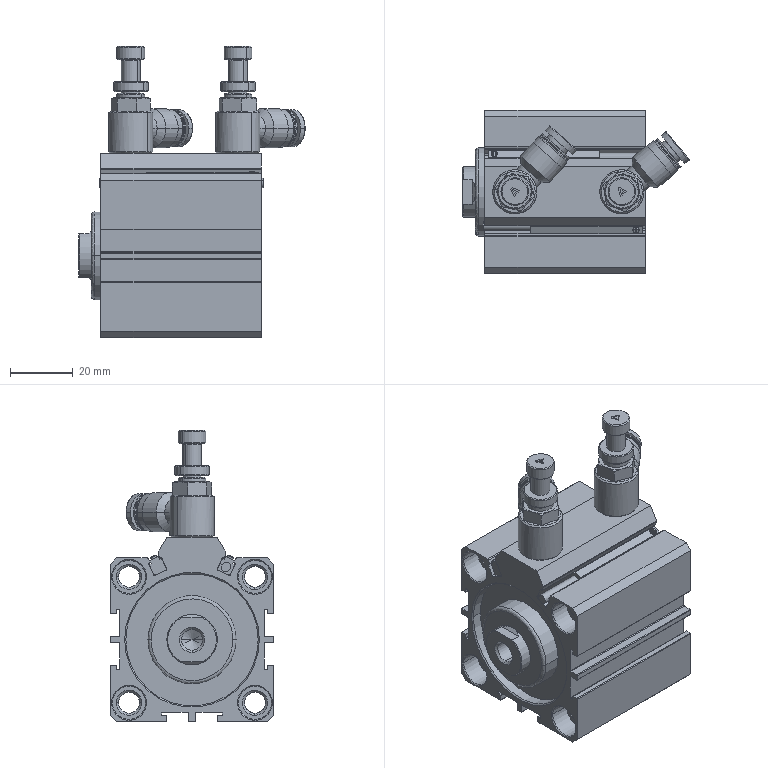Part | SolidWorks | features BaseBody 6, MoveFace 2 | 6 solids | 525 faces | box 71.881 x 52 x 92.5 mm | volume 126457 mm3 | cylinder 194 | plane 190 | cone 123 | spline 18 | commonest cylinder face diameters 0.4 x50 10.5 x16 6 x12 0.8 x10 6.647 x10 8.8 x8